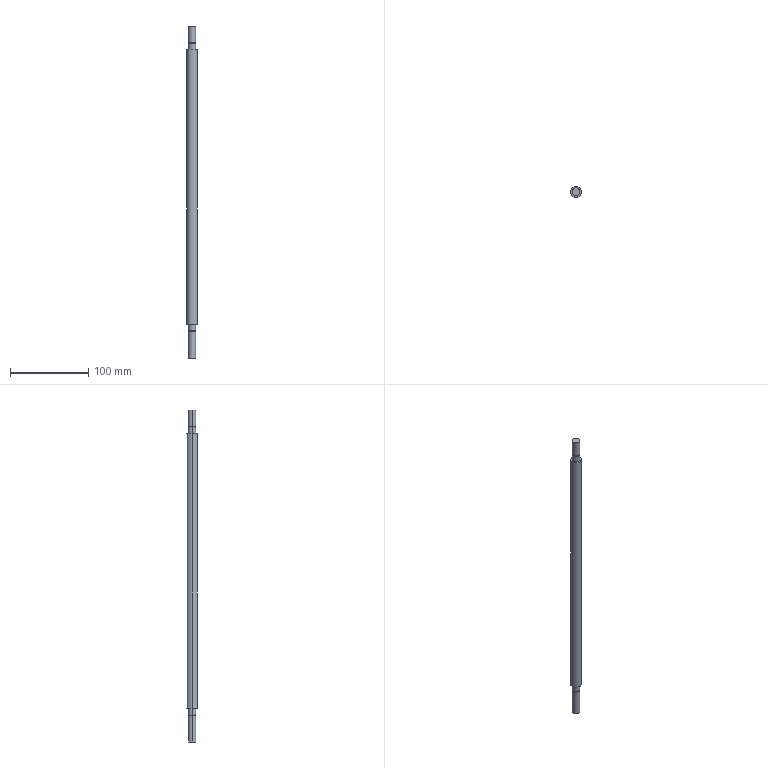Part | STEP file | 602-09-0047 | 1 solid | 24 faces | box 14 x 14 x 425 mm | volume 59824 mm3 | cylinder 14 | plane 10 | commonest cylinder face diameters 10 x8 9.6 x4 14 x2
STEP:
#1=CARTESIAN_POINT('',(0.,0.,0.));
#2=DIRECTION('',(0.,0.,1.));
#3=DIRECTION('',(1.,0.,0.));
#4=AXIS2_PLACEMENT_3D('',#1,#2,#3);
#5=CARTESIAN_POINT('',(-5.,0.,-43.));
#6=VERTEX_POINT('',#5);
#7=CARTESIAN_POINT('',(-3.,4.,-43.));
#8=VERTEX_POINT('',#7);
#9=CARTESIAN_POINT('',(0.,0.,-43.));
#10=DIRECTION('',(0.,0.,-1.));
#11=DIRECTION('',(-1.,0.,0.));
#12=AXIS2_PLACEMENT_3D('',#9,#10,#11);
#13=CIRCLE('',#12,5.);
#14=CARTESIAN_POINT('',(0.,0.,-43.));
#15=DIRECTION('',(0.,0.,1.));
#16=DIRECTION('',(1.,0.,0.));
#17=AXIS2_PLACEMENT_3D('',#14,#15,#16);
#18=CYLINDRICAL_SURFACE('',#17,5.);
#19=CARTESIAN_POINT('',(3.142,0.));
#20=DIRECTION('',(-1.,0.));
#21=VECTOR('',#20,1.);
#22=LINE('',#19,#21);
#23=(GEOMETRIC_REPRESENTATION_CONTEXT(2)PARAMETRIC_REPRESENTATION_CONTEXT()REPRESENTATION_CONTEXT('',''));
#24=DEFINITIONAL_REPRESENTATION('',(#22),#23);
#25=PCURVE('',#18,#24);
#26=CARTESIAN_POINT('',(0.,0.,-43.));
#27=DIRECTION('',(0.,0.,-1.));
#28=DIRECTION('',(-1.,0.,0.));
#29=AXIS2_PLACEMENT_3D('',#26,#27,#28);
#30=PLANE('',#29);
#31=CARTESIAN_POINT('',(0.,0.));
#32=DIRECTION('',(1.,0.));
#33=AXIS2_PLACEMENT_2D('',#31,#32);
#34=CIRCLE('',#33,5.);
#35=(GEOMETRIC_REPRESENTATION_CONTEXT(2)PARAMETRIC_REPRESENTATION_CONTEXT()REPRESENTATION_CONTEXT('',''));
#36=DEFINITIONAL_REPRESENTATION('',(#34),#35);
#37=PCURVE('',#30,#36);
#38=SURFACE_CURVE('',#13,(#25,#37),.PCURVE_S1.);
#39=EDGE_CURVE('',#6,#8,#38,.T.);
#40=ORIENTED_EDGE('',*,*,#39,.F.);
#41=CARTESIAN_POINT('',(-5.,0.,-9.1));
#42=VERTEX_POINT('',#41);
#43=CARTESIAN_POINT('',(-5.,0.,-43.));
#44=DIRECTION('',(0.,0.,1.));
#45=VECTOR('',#44,1.);
#46=LINE('',#43,#45);
#47=CARTESIAN_POINT('',(3.142,0.));
#48=DIRECTION('',(0.,1.));
#49=VECTOR('',#48,1.);
#50=LINE('',#47,#49);
#51=(GEOMETRIC_REPRESENTATION_CONTEXT(2)PARAMETRIC_REPRESENTATION_CONTEXT()REPRESENTATION_CONTEXT('',''));
#52=DEFINITIONAL_REPRESENTATION('',(#50),#51);
#53=PCURVE('',#18,#52);
#54=CARTESIAN_POINT('',(0.,0.,-43.));
#55=DIRECTION('',(0.,0.,1.));
#56=DIRECTION('',(1.,0.,0.));
#57=AXIS2_PLACEMENT_3D('',#54,#55,#56);
#58=CYLINDRICAL_SURFACE('',#57,5.);
#59=CARTESIAN_POINT('',(3.142,0.));
#60=DIRECTION('',(0.,1.));
#61=VECTOR('',#60,1.);
#62=LINE('',#59,#61);
#63=(GEOMETRIC_REPRESENTATION_CONTEXT(2)PARAMETRIC_REPRESENTATION_CONTEXT()REPRESENTATION_CONTEXT('',''));
#64=DEFINITIONAL_REPRESENTATION('',(#62),#63);
#65=PCURVE('',#58,#64);
#66=SURFACE_CURVE('',#46,(#53,#65),.PCURVE_S1.);
#67=EDGE_CURVE('',#6,#42,#66,.T.);
#68=ORIENTED_EDGE('',*,*,#67,.T.);
#69=CARTESIAN_POINT('',(5.,0.,-9.1));
#70=VERTEX_POINT('',#69);
#71=CARTESIAN_POINT('',(0.,0.,-9.1));
#72=DIRECTION('',(0.,0.,-1.));
#73=DIRECTION('',(-1.,0.,0.));
#74=AXIS2_PLACEMENT_3D('',#71,#72,#73);
#75=CIRCLE('',#74,5.);
#76=CARTESIAN_POINT('',(3.142,33.9));
#77=DIRECTION('',(-1.,0.));
#78=VECTOR('',#77,1.);
#79=LINE('',#76,#78);
#80=(GEOMETRIC_REPRESENTATION_CONTEXT(2)PARAMETRIC_REPRESENTATION_CONTEXT()REPRESENTATION_CONTEXT('',''));
#81=DEFINITIONAL_REPRESENTATION('',(#79),#80);
#82=PCURVE('',#18,#81);
#83=CARTESIAN_POINT('',(0.,0.,-9.1));
#84=DIRECTION('',(0.,0.,-1.));
#85=DIRECTION('',(-1.,0.,0.));
#86=AXIS2_PLACEMENT_3D('',#83,#84,#85);
#87=PLANE('',#86);
#88=CARTESIAN_POINT('',(0.,0.));
#89=DIRECTION('',(1.,0.));
#90=AXIS2_PLACEMENT_2D('',#88,#89);
#91=CIRCLE('',#90,5.);
#92=(GEOMETRIC_REPRESENTATION_CONTEXT(2)PARAMETRIC_REPRESENTATION_CONTEXT()REPRESENTATION_CONTEXT('',''));
#93=DEFINITIONAL_REPRESENTATION('',(#91),#92);
#94=PCURVE('',#87,#93);
#95=SURFACE_CURVE('',#75,(#82,#94),.PCURVE_S1.);
#96=EDGE_CURVE('',#42,#70,#95,.T.);
#97=ORIENTED_EDGE('',*,*,#96,.T.);
#98=CARTESIAN_POINT('',(5.,0.,-43.));
#99=VERTEX_POINT('',#98);
#100=CARTESIAN_POINT('',(5.,0.,-43.));
#101=DIRECTION('',(0.,0.,1.));
#102=VECTOR('',#101,1.);
#103=LINE('',#100,#102);
#104=CARTESIAN_POINT('',(0.,0.));
#105=DIRECTION('',(0.,1.));
#106=VECTOR('',#105,1.);
#107=LINE('',#104,#106);
#108=(GEOMETRIC_REPRESENTATION_CONTEXT(2)PARAMETRIC_REPRESENTATION_CONTEXT()REPRESENTATION_CONTEXT('',''));
#109=DEFINITIONAL_REPRESENTATION('',(#107),#108);
#110=PCURVE('',#18,#109);
#111=CARTESIAN_POINT('',(6.283,0.));
#112=DIRECTION('',(0.,1.));
#113=VECTOR('',#112,1.);
#114=LINE('',#111,#113);
#115=(GEOMETRIC_REPRESENTATION_CONTEXT(2)PARAMETRIC_REPRESENTATION_CONTEXT()REPRESENTATION_CONTEXT('',''));
#116=DEFINITIONAL_REPRESENTATION('',(#114),#115);
#117=PCURVE('',#58,#116);
#118=SURFACE_CURVE('',#103,(#110,#117),.PCURVE_S1.);
#119=EDGE_CURVE('',#99,#70,#118,.T.);
#120=ORIENTED_EDGE('',*,*,#119,.F.);
#121=CARTESIAN_POINT('',(3.,4.,-43.));
#122=VERTEX_POINT('',#121);
#123=CARTESIAN_POINT('',(0.,0.,-43.));
#124=DIRECTION('',(0.,0.,-1.));
#125=DIRECTION('',(-1.,0.,0.));
#126=AXIS2_PLACEMENT_3D('',#123,#124,#125);
#127=CIRCLE('',#126,5.);
#128=CARTESIAN_POINT('',(3.142,0.));
#129=DIRECTION('',(-1.,0.));
#130=VECTOR('',#129,1.);
#131=LINE('',#128,#130);
#132=(GEOMETRIC_REPRESENTATION_CONTEXT(2)PARAMETRIC_REPRESENTATION_CONTEXT()REPRESENTATION_CONTEXT('',''));
#133=DEFINITIONAL_REPRESENTATION('',(#131),#132);
#134=PCURVE('',#18,#133);
#135=CARTESIAN_POINT('',(0.,0.));
#136=DIRECTION('',(1.,0.));
#137=AXIS2_PLACEMENT_2D('',#135,#136);
#138=CIRCLE('',#137,5.);
#139=(GEOMETRIC_REPRESENTATION_CONTEXT(2)PARAMETRIC_REPRESENTATION_CONTEXT()REPRESENTATION_CONTEXT('',''));
#140=DEFINITIONAL_REPRESENTATION('',(#138),#139);
#141=PCURVE('',#30,#140);
#142=SURFACE_CURVE('',#127,(#134,#141),.PCURVE_S1.);
#143=EDGE_CURVE('',#122,#99,#142,.T.);
#144=ORIENTED_EDGE('',*,*,#143,.F.);
#145=CARTESIAN_POINT('',(3.,4.,-23.));
#146=VERTEX_POINT('',#145);
#147=CARTESIAN_POINT('',(3.,4.,-23.));
#148=DIRECTION('',(0.,0.,-1.));
#149=VECTOR('',#148,1.);
#150=LINE('',#147,#149);
#151=CARTESIAN_POINT('',(0.9273,20.));
#152=DIRECTION('',(0.,-1.));
#153=VECTOR('',#152,1.);
#154=LINE('',#151,#153);
#155=(GEOMETRIC_REPRESENTATION_CONTEXT(2)PARAMETRIC_REPRESENTATION_CONTEXT()REPRESENTATION_CONTEXT('',''));
#156=DEFINITIONAL_REPRESENTATION('',(#154),#155);
#157=PCURVE('',#18,#156);
#158=CARTESIAN_POINT('',(3.,4.,-23.));
#159=DIRECTION('',(0.,-1.,0.));
#160=DIRECTION('',(0.,0.,-1.));
#161=AXIS2_PLACEMENT_3D('',#158,#159,#160);
#162=PLANE('',#161);
#163=CARTESIAN_POINT('',(0.,0.));
#164=DIRECTION('',(1.,0.));
#165=VECTOR('',#164,1.);
#166=LINE('',#163,#165);
#167=(GEOMETRIC_REPRESENTATION_CONTEXT(2)PARAMETRIC_REPRESENTATION_CONTEXT()REPRESENTATION_CONTEXT('',''));
#168=DEFINITIONAL_REPRESENTATION('',(#166),#167);
#169=PCURVE('',#162,#168);
#170=SURFACE_CURVE('',#150,(#157,#169),.PCURVE_S1.);
#171=EDGE_CURVE('',#146,#122,#170,.T.);
#172=ORIENTED_EDGE('',*,*,#171,.F.);
#173=CARTESIAN_POINT('',(-3.,4.,-23.));
#174=VERTEX_POINT('',#173);
#175=CARTESIAN_POINT('',(0.,0.,-23.));
#176=DIRECTION('',(0.,0.,-1.));
#177=DIRECTION('',(-1.,0.,0.));
#178=AXIS2_PLACEMENT_3D('',#175,#176,#177);
#179=CIRCLE('',#178,5.);
#180=CARTESIAN_POINT('',(3.142,20.));
#181=DIRECTION('',(-1.,0.));
#182=VECTOR('',#181,1.);
#183=LINE('',#180,#182);
#184=(GEOMETRIC_REPRESENTATION_CONTEXT(2)PARAMETRIC_REPRESENTATION_CONTEXT()REPRESENTATION_CONTEXT('',''));
#185=DEFINITIONAL_REPRESENTATION('',(#183),#184);
#186=PCURVE('',#18,#185);
#187=CARTESIAN_POINT('',(0.,0.,-23.));
#188=DIRECTION('',(0.,0.,-1.));
#189=DIRECTION('',(-1.,0.,0.));
#190=AXIS2_PLACEMENT_3D('',#187,#188,#189);
#191=PLANE('',#190);
#192=CARTESIAN_POINT('',(0.,0.));
#193=DIRECTION('',(1.,0.));
#194=AXIS2_PLACEMENT_2D('',#192,#193);
#195=CIRCLE('',#194,5.);
#196=(GEOMETRIC_REPRESENTATION_CONTEXT(2)PARAMETRIC_REPRESENTATION_CONTEXT()REPRESENTATION_CONTEXT('',''));
#197=DEFINITIONAL_REPRESENTATION('',(#195),#196);
#198=PCURVE('',#191,#197);
#199=SURFACE_CURVE('',#179,(#186,#198),.PCURVE_S1.);
#200=EDGE_CURVE('',#174,#146,#199,.T.);
#201=ORIENTED_EDGE('',*,*,#200,.F.);
#202=CARTESIAN_POINT('',(-3.,4.,-23.));
#203=DIRECTION('',(0.,0.,-1.));
#204=VECTOR('',#203,1.);
#205=LINE('',#202,#204);
#206=CARTESIAN_POINT('',(2.214,20.));
#207=DIRECTION('',(0.,-1.));
#208=VECTOR('',#207,1.);
#209=LINE('',#206,#208);
#210=(GEOMETRIC_REPRESENTATION_CONTEXT(2)PARAMETRIC_REPRESENTATION_CONTEXT()REPRESENTATION_CONTEXT('',''));
#211=DEFINITIONAL_REPRESENTATION('',(#209),#210);
#212=PCURVE('',#18,#211);
#213=CARTESIAN_POINT('',(0.,-6.));
#214=DIRECTION('',(1.,0.));
#215=VECTOR('',#214,1.);
#216=LINE('',#213,#215);
#217=(GEOMETRIC_REPRESENTATION_CONTEXT(2)PARAMETRIC_REPRESENTATION_CONTEXT()REPRESENTATION_CONTEXT('',''));
#218=DEFINITIONAL_REPRESENTATION('',(#216),#217);
#219=PCURVE('',#162,#218);
#220=SURFACE_CURVE('',#205,(#212,#219),.PCURVE_S1.);
#221=EDGE_CURVE('',#174,#8,#220,.T.);
#222=ORIENTED_EDGE('',*,*,#221,.T.);
#223=EDGE_LOOP('',(#40,#68,#97,#120,#144,#172,#201,#222));
#224=FACE_BOUND('',#223,.T.);
#225=ADVANCED_FACE('',(#224),#18,.T.);
#226=CARTESIAN_POINT('',(-4.8,0.,-9.1));
#227=VERTEX_POINT('',#226);
#228=CARTESIAN_POINT('',(4.8,0.,-9.1));
#229=VERTEX_POINT('',#228);
#230=CARTESIAN_POINT('',(0.,0.,-9.1));
#231=DIRECTION('',(0.,0.,-1.));
#232=DIRECTION('',(-1.,0.,0.));
#233=AXIS2_PLACEMENT_3D('',#230,#231,#232);
#234=CIRCLE('',#233,4.8);
#235=CARTESIAN_POINT('',(0.,0.,-9.1));
#236=DIRECTION('',(0.,0.,1.));
#237=DIRECTION('',(1.,0.,0.));
#238=AXIS2_PLACEMENT_3D('',#235,#236,#237);
#239=CYLINDRICAL_SURFACE('',#238,4.8);
#240=CARTESIAN_POINT('',(3.142,0.));
#241=DIRECTION('',(-1.,0.));
#242=VECTOR('',#241,1.);
#243=LINE('',#240,#242);
#244=(GEOMETRIC_REPRESENTATION_CONTEXT(2)PARAMETRIC_REPRESENTATION_CONTEXT()REPRESENTATION_CONTEXT('',''));
#245=DEFINITIONAL_REPRESENTATION('',(#243),#244);
#246=PCURVE('',#239,#245);
#247=CARTESIAN_POINT('',(0.,0.));
#248=DIRECTION('',(1.,0.));
#249=AXIS2_PLACEMENT_2D('',#247,#248);
#250=CIRCLE('',#249,4.8);
#251=(GEOMETRIC_REPRESENTATION_CONTEXT(2)PARAMETRIC_REPRESENTATION_CONTEXT()REPRESENTATION_CONTEXT('',''));
#252=DEFINITIONAL_REPRESENTATION('',(#250),#251);
#253=PCURVE('',#87,#252);
#254=SURFACE_CURVE('',#234,(#246,#253),.PCURVE_S1.);
#255=EDGE_CURVE('',#227,#229,#254,.T.);
#256=ORIENTED_EDGE('',*,*,#255,.F.);
#257=CARTESIAN_POINT('',(-4.8,0.,-8.));
#258=VERTEX_POINT('',#257);
#259=CARTESIAN_POINT('',(-4.8,0.,-9.1));
#260=DIRECTION('',(0.,0.,1.));
#261=VECTOR('',#260,1.);
#262=LINE('',#259,#261);
#263=CARTESIAN_POINT('',(3.142,0.));
#264=DIRECTION('',(0.,1.));
#265=VECTOR('',#264,1.);
#266=LINE('',#263,#265);
#267=(GEOMETRIC_REPRESENTATION_CONTEXT(2)PARAMETRIC_REPRESENTATION_CONTEXT()REPRESENTATION_CONTEXT('',''));
#268=DEFINITIONAL_REPRESENTATION('',(#266),#267);
#269=PCURVE('',#239,#268);
#270=CARTESIAN_POINT('',(0.,0.,-9.1));
#271=DIRECTION('',(0.,0.,1.));
#272=DIRECTION('',(1.,0.,0.));
#273=AXIS2_PLACEMENT_3D('',#270,#271,#272);
#274=CYLINDRICAL_SURFACE('',#273,4.8);
#275=CARTESIAN_POINT('',(3.142,0.));
#276=DIRECTION('',(0.,1.));
#277=VECTOR('',#276,1.);
#278=LINE('',#275,#277);
#279=(GEOMETRIC_REPRESENTATION_CONTEXT(2)PARAMETRIC_REPRESENTATION_CONTEXT()REPRESENTATION_CONTEXT('',''));
#280=DEFINITIONAL_REPRESENTATION('',(#278),#279);
#281=PCURVE('',#274,#280);
#282=SURFACE_CURVE('',#262,(#269,#281),.PCURVE_S1.);
#283=EDGE_CURVE('',#227,#258,#282,.T.);
#284=ORIENTED_EDGE('',*,*,#283,.T.);
#285=CARTESIAN_POINT('',(4.8,0.,-8.));
#286=VERTEX_POINT('',#285);
#287=CARTESIAN_POINT('',(0.,0.,-8.));
#288=DIRECTION('',(0.,0.,-1.));
#289=DIRECTION('',(-1.,0.,0.));
#290=AXIS2_PLACEMENT_3D('',#287,#288,#289);
#291=CIRCLE('',#290,4.8);
#292=CARTESIAN_POINT('',(3.142,1.1));
#293=DIRECTION('',(-1.,0.));
#294=VECTOR('',#293,1.);
#295=LINE('',#292,#294);
#296=(GEOMETRIC_REPRESENTATION_CONTEXT(2)PARAMETRIC_REPRESENTATION_CONTEXT()REPRESENTATION_CONTEXT('',''));
#297=DEFINITIONAL_REPRESENTATION('',(#295),#296);
#298=PCURVE('',#239,#297);
#299=CARTESIAN_POINT('',(0.,0.,-8.));
#300=DIRECTION('',(0.,0.,-1.));
#301=DIRECTION('',(-1.,0.,0.));
#302=AXIS2_PLACEMENT_3D('',#299,#300,#301);
#303=PLANE('',#302);
#304=CARTESIAN_POINT('',(0.,0.));
#305=DIRECTION('',(1.,0.));
#306=AXIS2_PLACEMENT_2D('',#304,#305);
#307=CIRCLE('',#306,4.8);
#308=(GEOMETRIC_REPRESENTATION_CONTEXT(2)PARAMETRIC_REPRESENTATION_CONTEXT()REPRESENTATION_CONTEXT('',''));
#309=DEFINITIONAL_REPRESENTATION('',(#307),#308);
#310=PCURVE('',#303,#309);
#311=SURFACE_CURVE('',#291,(#298,#310),.PCURVE_S1.);
#312=EDGE_CURVE('',#258,#286,#311,.T.);
#313=ORIENTED_EDGE('',*,*,#312,.T.);
#314=CARTESIAN_POINT('',(4.8,0.,-9.1));
#315=DIRECTION('',(0.,0.,1.));
#316=VECTOR('',#315,1.);
#317=LINE('',#314,#316);
#318=CARTESIAN_POINT('',(0.,0.));
#319=DIRECTION('',(0.,1.));
#320=VECTOR('',#319,1.);
#321=LINE('',#318,#320);
#322=(GEOMETRIC_REPRESENTATION_CONTEXT(2)PARAMETRIC_REPRESENTATION_CONTEXT()REPRESENTATION_CONTEXT('',''));
#323=DEFINITIONAL_REPRESENTATION('',(#321),#322);
#324=PCURVE('',#239,#323);
#325=CARTESIAN_POINT('',(6.283,0.));
#326=DIRECTION('',(0.,1.));
#327=VECTOR('',#326,1.);
#328=LINE('',#325,#327);
#329=(GEOMETRIC_REPRESENTATION_CONTEXT(2)PARAMETRIC_REPRESENTATION_CONTEXT()REPRESENTATION_CONTEXT('',''));
#330=DEFINITIONAL_REPRESENTATION('',(#328),#329);
#331=PCURVE('',#274,#330);
#332=SURFACE_CURVE('',#317,(#324,#331),.PCURVE_S1.);
#333=EDGE_CURVE('',#229,#286,#332,.T.);
#334=ORIENTED_EDGE('',*,*,#333,.F.);
#335=EDGE_LOOP('',(#256,#284,#313,#334));
#336=FACE_BOUND('',#335,.T.);
#337=ADVANCED_FACE('',(#336),#239,.T.);
#338=CARTESIAN_POINT('',(5.,0.,382.));
#339=VERTEX_POINT('',#338);
#340=CARTESIAN_POINT('',(-5.,0.,382.));
#341=VERTEX_POINT('',#340);
#342=CARTESIAN_POINT('',(0.,0.,382.));
#343=DIRECTION('',(0.,0.,1.));
#344=DIRECTION('',(1.,0.,0.));
#345=AXIS2_PLACEMENT_3D('',#342,#343,#344);
#346=CIRCLE('',#345,5.);
#347=CARTESIAN_POINT('',(0.,0.,382.));
#348=DIRECTION('',(0.,0.,-1.));
#349=DIRECTION('',(-1.,0.,0.));
#350=AXIS2_PLACEMENT_3D('',#347,#348,#349);
#351=CYLINDRICAL_SURFACE('',#350,5.);
#352=CARTESIAN_POINT('',(3.142,0.));
#353=DIRECTION('',(-1.,0.));
#354=VECTOR('',#353,1.);
#355=LINE('',#352,#354);
#356=(GEOMETRIC_REPRESENTATION_CONTEXT(2)PARAMETRIC_REPRESENTATION_CONTEXT()REPRESENTATION_CONTEXT('',''));
#357=DEFINITIONAL_REPRESENTATION('',(#355),#356);
#358=PCURVE('',#351,#357);
#359=CARTESIAN_POINT('',(0.,0.,382.));
#360=DIRECTION('',(0.,0.,1.));
#361=DIRECTION('',(1.,0.,0.));
#362=AXIS2_PLACEMENT_3D('',#359,#360,#361);
#363=PLANE('',#362);
#364=CARTESIAN_POINT('',(0.,0.));
#365=DIRECTION('',(1.,0.));
#366=AXIS2_PLACEMENT_2D('',#364,#365);
#367=CIRCLE('',#366,5.);
#368=(GEOMETRIC_REPRESENTATION_CONTEXT(2)PARAMETRIC_REPRESENTATION_CONTEXT()REPRESENTATION_CONTEXT('',''));
#369=DEFINITIONAL_REPRESENTATION('',(#367),#368);
#370=PCURVE('',#363,#369);
#371=SURFACE_CURVE('',#346,(#358,#370),.PCURVE_S1.);
#372=EDGE_CURVE('',#339,#341,#371,.T.);
#373=ORIENTED_EDGE('',*,*,#372,.F.);
#374=CARTESIAN_POINT('',(5.,0.,361.1));
#375=VERTEX_POINT('',#374);
#376=CARTESIAN_POINT('',(5.,0.,382.));
#377=DIRECTION('',(0.,0.,-1.));
#378=VECTOR('',#377,1.);
#379=LINE('',#376,#378);
#380=CARTESIAN_POINT('',(3.142,0.));
#381=DIRECTION('',(0.,1.));
#382=VECTOR('',#381,1.);
#383=LINE('',#380,#382);
#384=(GEOMETRIC_REPRESENTATION_CONTEXT(2)PARAMETRIC_REPRESENTATION_CONTEXT()REPRESENTATION_CONTEXT('',''));
#385=DEFINITIONAL_REPRESENTATION('',(#383),#384);
#386=PCURVE('',#351,#385);
#387=CARTESIAN_POINT('',(0.,0.,382.));
#388=DIRECTION('',(0.,0.,-1.));
#389=DIRECTION('',(-1.,0.,0.));
#390=AXIS2_PLACEMENT_3D('',#387,#388,#389);
#391=CYLINDRICAL_SURFACE('',#390,5.);
#392=CARTESIAN_POINT('',(3.142,0.));
#393=DIRECTION('',(0.,1.));
#394=VECTOR('',#393,1.);
#395=LINE('',#392,#394);
#396=(GEOMETRIC_REPRESENTATION_CONTEXT(2)PARAMETRIC_REPRESENTATION_CONTEXT()REPRESENTATION_CONTEXT('',''));
#397=DEFINITIONAL_REPRESENTATION('',(#395),#396);
#398=PCURVE('',#391,#397);
#399=SURFACE_CURVE('',#379,(#386,#398),.PCURVE_S1.);
#400=EDGE_CURVE('',#339,#375,#399,.T.);
#401=ORIENTED_EDGE('',*,*,#400,.T.);
#402=CARTESIAN_POINT('',(-5.,0.,361.1));
#403=VERTEX_POINT('',#402);
#404=CARTESIAN_POINT('',(0.,0.,361.1));
#405=DIRECTION('',(0.,0.,1.));
#406=DIRECTION('',(1.,0.,0.));
#407=AXIS2_PLACEMENT_3D('',#404,#405,#406);
#408=CIRCLE('',#407,5.);
#409=CARTESIAN_POINT('',(3.142,20.9));
#410=DIRECTION('',(-1.,0.));
#411=VECTOR('',#410,1.);
#412=LINE('',#409,#411);
#413=(GEOMETRIC_REPRESENTATION_CONTEXT(2)PARAMETRIC_REPRESENTATION_CONTEXT()REPRESENTATION_CONTEXT('',''));
#414=DEFINITIONAL_REPRESENTATION('',(#412),#413);
#415=PCURVE('',#351,#414);
#416=CARTESIAN_POINT('',(0.,0.,361.1));
#417=DIRECTION('',(0.,0.,1.));
#418=DIRECTION('',(1.,0.,0.));
#419=AXIS2_PLACEMENT_3D('',#416,#417,#418);
#420=PLANE('',#419);
#421=CARTESIAN_POINT('',(0.,0.));
#422=DIRECTION('',(1.,0.));
#423=AXIS2_PLACEMENT_2D('',#421,#422);
#424=CIRCLE('',#423,5.);
#425=(GEOMETRIC_REPRESENTATION_CONTEXT(2)PARAMETRIC_REPRESENTATION_CONTEXT()REPRESENTATION_CONTEXT('',''));
#426=DEFINITIONAL_REPRESENTATION('',(#424),#425);
#427=PCURVE('',#420,#426);
#428=SURFACE_CURVE('',#408,(#415,#427),.PCURVE_S1.);
#429=EDGE_CURVE('',#375,#403,#428,.T.);
#430=ORIENTED_EDGE('',*,*,#429,.T.);
#431=CARTESIAN_POINT('',(-5.,0.,382.));
#432=DIRECTION('',(0.,0.,-1.));
#433=VECTOR('',#432,1.);
#434=LINE('',#431,#433);
#435=CARTESIAN_POINT('',(0.,0.));
#436=DIRECTION('',(0.,1.));
#437=VECTOR('',#436,1.);
#438=LINE('',#435,#437);
#439=(GEOMETRIC_REPRESENTATION_CONTEXT(2)PARAMETRIC_REPRESENTATION_CONTEXT()REPRESENTATION_CONTEXT('',''));
#440=DEFINITIONAL_REPRESENTATION('',(#438),#439);
#441=PCURVE('',#351,#440);
#442=CARTESIAN_POINT('',(6.283,0.));
#443=DIRECTION('',(0.,1.));
#444=VECTOR('',#443,1.);
#445=LINE('',#442,#444);
#446=(GEOMETRIC_REPRESENTATION_CONTEXT(2)PARAMETRIC_REPRESENTATION_CONTEXT()REPRESENTATION_CONTEXT('',''));
#447=DEFINITIONAL_REPRESENTATION('',(#445),#446);
#448=PCURVE('',#391,#447);
#449=SURFACE_CURVE('',#434,(#441,#448),.PCURVE_S1.);
#450=EDGE_CURVE('',#341,#403,#449,.T.);
#451=ORIENTED_EDGE('',*,*,#450,.F.);
#452=EDGE_LOOP('',(#373,#401,#430,#451));
#453=FACE_BOUND('',#452,.T.);
#454=ADVANCED_FACE('',(#453),#351,.T.);
#455=CARTESIAN_POINT('',(4.8,0.,361.1));
#456=VERTEX_POINT('',#455);
#457=CARTESIAN_POINT('',(-4.8,0.,361.1));
#458=VERTEX_POINT('',#457);
#459=CARTESIAN_POINT('',(0.,0.,361.1));
#460=DIRECTION('',(0.,0.,1.));
#461=DIRECTION('',(1.,0.,0.));
#462=AXIS2_PLACEMENT_3D('',#459,#460,#461);
#463=CIRCLE('',#462,4.8);
#464=CARTESIAN_POINT('',(0.,0.,361.1));
#465=DIRECTION('',(0.,0.,-1.));
#466=DIRECTION('',(-1.,0.,0.));
#467=AXIS2_PLACEMENT_3D('',#464,#465,#466);
#468=CYLINDRICAL_SURFACE('',#467,4.8);
#469=CARTESIAN_POINT('',(3.142,0.));
#470=DIRECTION('',(-1.,0.));
#471=VECTOR('',#470,1.);
#472=LINE('',#469,#471);
#473=(GEOMETRIC_REPRESENTATION_CONTEXT(2)PARAMETRIC_REPRESENTATION_CONTEXT()REPRESENTATION_CONTEXT('',''));
#474=DEFINITIONAL_REPRESENTATION('',(#472),#473);
#475=PCURVE('',#468,#474);
#476=CARTESIAN_POINT('',(0.,0.));
#477=DIRECTION('',(1.,0.));
#478=AXIS2_PLACEMENT_2D('',#476,#477);
#479=CIRCLE('',#478,4.8);
#480=(GEOMETRIC_REPRESENTATION_CONTEXT(2)PARAMETRIC_REPRESENTATION_CONTEXT()REPRESENTATION_CONTEXT('',''));
#481=DEFINITIONAL_REPRESENTATION('',(#479),#480);
#482=PCURVE('',#420,#481);
#483=SURFACE_CURVE('',#463,(#475,#482),.PCURVE_S1.);
#484=EDGE_CURVE('',#456,#458,#483,.T.);
#485=ORIENTED_EDGE('',*,*,#484,.F.);
#486=CARTESIAN_POINT('',(4.8,0.,360.));
#487=VERTEX_POINT('',#486);
#488=CARTESIAN_POINT('',(4.8,0.,361.1));
#489=DIRECTION('',(0.,0.,-1.));
#490=VECTOR('',#489,1.);
#491=LINE('',#488,#490);
#492=CARTESIAN_POINT('',(3.142,0.));
#493=DIRECTION('',(0.,1.));
#494=VECTOR('',#493,1.);
#495=LINE('',#492,#494);
#496=(GEOMETRIC_REPRESENTATION_CONTEXT(2)PARAMETRIC_REPRESENTATION_CONTEXT()REPRESENTATION_CONTEXT('',''));
#497=DEFINITIONAL_REPRESENTATION('',(#495),#496);
#498=PCURVE('',#468,#497);
#499=CARTESIAN_POINT('',(0.,0.,361.1));
#500=DIRECTION('',(0.,0.,-1.));
#501=DIRECTION('',(-1.,0.,0.));
#502=AXIS2_PLACEMENT_3D('',#499,#500,#501);
#503=CYLINDRICAL_SURFACE('',#502,4.8);
#504=CARTESIAN_POINT('',(3.142,0.));
#505=DIRECTION('',(0.,1.));
#506=VECTOR('',#505,1.);
#507=LINE('',#504,#506);
#508=(GEOMETRIC_REPRESENTATION_CONTEXT(2)PARAMETRIC_REPRESENTATION_CONTEXT()REPRESENTATION_CONTEXT('',''));
#509=DEFINITIONAL_REPRESENTATION('',(#507),#508);
#510=PCURVE('',#503,#509);
#511=SURFACE_CURVE('',#491,(#498,#510),.PCURVE_S1.);
#512=EDGE_CURVE('',#456,#487,#511,.T.);
#513=ORIENTED_EDGE('',*,*,#512,.T.);
#514=CARTESIAN_POINT('',(-4.8,0.,360.));
#515=VERTEX_POINT('',#514);
#516=CARTESIAN_POINT('',(0.,0.,360.));
#517=DIRECTION('',(0.,0.,1.));
#518=DIRECTION('',(1.,0.,0.));
#519=AXIS2_PLACEMENT_3D('',#516,#517,#518);
#520=CIRCLE('',#519,4.8);
#521=CARTESIAN_POINT('',(3.142,1.1));
#522=DIRECTION('',(-1.,0.));
#523=VECTOR('',#522,1.);
#524=LINE('',#521,#523);
#525=(GEOMETRIC_REPRESENTATION_CONTEXT(2)PARAMETRIC_REPRESENTATION_CONTEXT()REPRESENTATION_CONTEXT('',''));
#526=DEFINITIONAL_REPRESENTATION('',(#524),#525);
#527=PCURVE('',#468,#526);
#528=CARTESIAN_POINT('',(0.,0.,360.));
#529=DIRECTION('',(0.,0.,1.));
#530=DIRECTION('',(1.,0.,0.));
#531=AXIS2_PLACEMENT_3D('',#528,#529,#530);
#532=PLANE('',#531);
#533=CARTESIAN_POINT('',(0.,0.));
#534=DIRECTION('',(1.,0.));
#535=AXIS2_PLACEMENT_2D('',#533,#534);
#536=CIRCLE('',#535,4.8);
#537=(GEOMETRIC_REPRESENTATION_CONTEXT(2)PARAMETRIC_REPRESENTATION_CONTEXT()REPRESENTATION_CONTEXT('',''));
#538=DEFINITIONAL_REPRESENTATION('',(#536),#537);
#539=PCURVE('',#532,#538);
#540=SURFACE_CURVE('',#520,(#527,#539),.PCURVE_S1.);
#541=EDGE_CURVE('',#487,#515,#540,.T.);
#542=ORIENTED_EDGE('',*,*,#541,.T.);
#543=CARTESIAN_POINT('',(-4.8,0.,361.1));
#544=DIRECTION('',(0.,0.,-1.));
#545=VECTOR('',#544,1.);
#546=LINE('',#543,#545);
#547=CARTESIAN_POINT('',(0.,0.));
#548=DIRECTION('',(0.,1.));
#549=VECTOR('',#548,1.);
#550=LINE('',#547,#549);
#551=(GEOMETRIC_REPRESENTATION_CONTEXT(2)PARAMETRIC_REPRESENTATION_CONTEXT()REPRESENTATION_CONTEXT('',''));
#552=DEFINITIONAL_REPRESENTATION('',(#550),#551);
#553=PCURVE('',#468,#552);
#554=CARTESIAN_POINT('',(6.283,0.));
#555=DIRECTION('',(0.,1.));
#556=VECTOR('',#555,1.);
#557=LINE('',#554,#556);
#558=(GEOMETRIC_REPRESENTATION_CONTEXT(2)PARAMETRIC_REPRESENTATION_CONTEXT()REPRESENTATION_CONTEXT('',''));
#559=DEFINITIONAL_REPRESENTATION('',(#557),#558);
#560=PCURVE('',#503,#559);
#561=SURFACE_CURVE('',#546,(#553,#560),.PCURVE_S1.);
#562=EDGE_CURVE('',#458,#515,#561,.T.);
#563=ORIENTED_EDGE('',*,*,#562,.F.);
#564=EDGE_LOOP('',(#485,#513,#542,#563));
#565=FACE_BOUND('',#564,.T.);
#566=ADVANCED_FACE('',(#565),#468,.T.);
#567=CARTESIAN_POINT('',(7.,0.,352.));
#568=VERTEX_POINT('',#567);
#569=CARTESIAN_POINT('',(-7.,0.,352.));
#570=VERTEX_POINT('',#569);
#571=CARTESIAN_POINT('',(0.,0.,352.));
#572=DIRECTION('',(0.,0.,1.));
#573=DIRECTION('',(1.,0.,0.));
#574=AXIS2_PLACEMENT_3D('',#571,#572,#573);
#575=CIRCLE('',#574,7.);
#576=CARTESIAN_POINT('',(0.,0.,352.));
#577=DIRECTION('',(0.,0.,-1.));
#578=DIRECTION('',(-1.,0.,0.));
#579=AXIS2_PLACEMENT_3D('',#576,#577,#578);
#580=CYLINDRICAL_SURFACE('',#579,7.);
#581=CARTESIAN_POINT('',(3.142,0.));
#582=DIRECTION('',(-1.,0.));
#583=VECTOR('',#582,1.);
#584=LINE('',#581,#583);
#585=(GEOMETRIC_REPRESENTATION_CONTEXT(2)PARAMETRIC_REPRESENTATION_CONTEXT()REPRESENTATION_CONTEXT('',''));
#586=DEFINITIONAL_REPRESENTATION('',(#584),#585);
#587=PCURVE('',#580,#586);
#588=CARTESIAN_POINT('',(0.,0.,352.));
#589=DIRECTION('',(0.,0.,1.));
#590=DIRECTION('',(1.,0.,0.));
#591=AXIS2_PLACEMENT_3D('',#588,#589,#590);
#592=PLANE('',#591);
#593=CARTESIAN_POINT('',(0.,0.));
#594=DIRECTION('',(1.,0.));
#595=AXIS2_PLACEMENT_2D('',#593,#594);
#596=CIRCLE('',#595,7.);
#597=(GEOMETRIC_REPRESENTATION_CONTEXT(2)PARAMETRIC_REPRESENTATION_CONTEXT()REPRESENTATION_CONTEXT('',''));
#598=DEFINITIONAL_REPRESENTATION('',(#596),#597);
#599=PCURVE('',#592,#598);
#600=SURFACE_CURVE('',#575,(#587,#599),.PCURVE_S1.);
#601=EDGE_CURVE('',#568,#570,#600,.T.);
#602=ORIENTED_EDGE('',*,*,#601,.F.);
#603=CARTESIAN_POINT('',(7.,0.,0.));
#604=VERTEX_POINT('',#603);
#605=CARTESIAN_POINT('',(7.,0.,352.));
#606=DIRECTION('',(0.,0.,-1.));
#607=VECTOR('',#606,1.);
#608=LINE('',#605,#607);
#609=CARTESIAN_POINT('',(3.142,0.));
#610=DIRECTION('',(0.,1.));
#611=VECTOR('',#610,1.);
#612=LINE('',#609,#611);
#613=(GEOMETRIC_REPRESENTATION_CONTEXT(2)PARAMETRIC_REPRESENTATION_CONTEXT()REPRESENTATION_CONTEXT('',''));
#614=DEFINITIONAL_REPRESENTATION('',(#612),#613);
#615=PCURVE('',#580,#614);
#616=CARTESIAN_POINT('',(0.,0.,352.));
#617=DIRECTION('',(0.,0.,-1.));
#618=DIRECTION('',(-1.,0.,0.));
#619=AXIS2_PLACEMENT_3D('',#616,#617,#618);
#620=CYLINDRICAL_SURFACE('',#619,7.);
#621=CARTESIAN_POINT('',(3.142,0.));
#622=DIRECTION('',(0.,1.));
#623=VECTOR('',#622,1.);
#624=LINE('',#621,#623);
#625=(GEOMETRIC_REPRESENTATION_CONTEXT(2)PARAMETRIC_REPRESENTATION_CONTEXT()REPRESENTATION_CONTEXT('',''));
#626=DEFINITIONAL_REPRESENTATION('',(#624),#625);
#627=PCURVE('',#620,#626);
#628=SURFACE_CURVE('',#608,(#615,#627),.PCURVE_S1.);
#629=EDGE_CURVE('',#568,#604,#628,.T.);
#630=ORIENTED_EDGE('',*,*,#629,.T.);
#631=CARTESIAN_POINT('',(-7.,0.,0.));
#632=VERTEX_POINT('',#631);
#633=CARTESIAN_POINT('',(0.,0.,0.));
#634=DIRECTION('',(0.,0.,1.));
#635=DIRECTION('',(1.,0.,0.));
#636=AXIS2_PLACEMENT_3D('',#633,#634,#635);
#637=CIRCLE('',#636,7.);
#638=CARTESIAN_POINT('',(3.142,352.));
#639=DIRECTION('',(-1.,0.));
#640=VECTOR('',#639,1.);
#641=LINE('',#638,#640);
#642=(GEOMETRIC_REPRESENTATION_CONTEXT(2)PARAMETRIC_REPRESENTATION_CONTEXT()REPRESENTATION_CONTEXT('',''));
#643=DEFINITIONAL_REPRESENTATION('',(#641),#642);
#644=PCURVE('',#580,#643);
#645=CARTESIAN_POINT('',(0.,0.,0.));
#646=DIRECTION('',(0.,0.,1.));
#647=DIRECTION('',(1.,0.,0.));
#648=AXIS2_PLACEMENT_3D('',#645,#646,#647);
#649=PLANE('',#648);
#650=CARTESIAN_POINT('',(0.,0.));
#651=DIRECTION('',(1.,0.));
#652=AXIS2_PLACEMENT_2D('',#650,#651);
#653=CIRCLE('',#652,7.);
#654=(GEOMETRIC_REPRESENTATION_CONTEXT(2)PARAMETRIC_REPRESENTATION_CONTEXT()REPRESENTATION_CONTEXT('',''));
#655=DEFINITIONAL_REPRESENTATION('',(#653),#654);
#656=PCURVE('',#649,#655);
#657=SURFACE_CURVE('',#637,(#644,#656),.PCURVE_S1.);
#658=EDGE_CURVE('',#604,#632,#657,.T.);
#659=ORIENTED_EDGE('',*,*,#658,.T.);
#660=CARTESIAN_POINT('',(-7.,0.,352.));
#661=DIRECTION('',(0.,0.,-1.));
#662=VECTOR('',#661,1.);
#663=LINE('',#660,#662);
#664=CARTESIAN_POINT('',(0.,0.));
#665=DIRECTION('',(0.,1.));
#666=VECTOR('',#665,1.);
#667=LINE('',#664,#666);
#668=(GEOMETRIC_REPRESENTATION_CONTEXT(2)PARAMETRIC_REPRESENTATION_CONTEXT()REPRESENTATION_CONTEXT('',''));
#669=DEFINITIONAL_REPRESENTATION('',(#667),#668);
#670=PCURVE('',#580,#669);
#671=CARTESIAN_POINT('',(6.283,0.));
#672=DIRECTION('',(0.,1.));
#673=VECTOR('',#672,1.);
#674=LINE('',#671,#673);
#675=(GEOMETRIC_REPRESENTATION_CONTEXT(2)PARAMETRIC_REPRESENTATION_CONTEXT()REPRESENTATION_CONTEXT('',''));
#676=DEFINITIONAL_REPRESENTATION('',(#674),#675);
#677=PCURVE('',#620,#676);
#678=SURFACE_CURVE('',#663,(#670,#677),.PCURVE_S1.);
#679=EDGE_CURVE('',#570,#632,#678,.T.);
#680=ORIENTED_EDGE('',*,*,#679,.F.);
#681=EDGE_LOOP('',(#602,#630,#659,#680));
#682=FACE_BOUND('',#681,.T.);
#683=ADVANCED_FACE('',(#682),#580,.T.);
#684=CARTESIAN_POINT('',(5.,0.,360.));
#685=VERTEX_POINT('',#684);
#686=CARTESIAN_POINT('',(-5.,0.,360.));
#687=VERTEX_POINT('',#686);
#688=CARTESIAN_POINT('',(0.,0.,360.));
#689=DIRECTION('',(0.,0.,1.));
#690=DIRECTION('',(1.,0.,0.));
#691=AXIS2_PLACEMENT_3D('',#688,#689,#690);
#692=CIRCLE('',#691,5.);
#693=CARTESIAN_POINT('',(0.,0.,382.));
#694=DIRECTION('',(0.,0.,-1.));
#695=DIRECTION('',(-1.,0.,0.));
#696=AXIS2_PLACEMENT_3D('',#693,#694,#695);
#697=CYLINDRICAL_SURFACE('',#696,5.);
#698=CARTESIAN_POINT('',(3.142,22.));
#699=DIRECTION('',(-1.,0.));
#700=VECTOR('',#699,1.);
#701=LINE('',#698,#700);
#702=(GEOMETRIC_REPRESENTATION_CONTEXT(2)PARAMETRIC_REPRESENTATION_CONTEXT()REPRESENTATION_CONTEXT('',''));
#703=DEFINITIONAL_REPRESENTATION('',(#701),#702);
#704=PCURVE('',#697,#703);
#705=CARTESIAN_POINT('',(0.,0.));
#706=DIRECTION('',(1.,0.));
#707=AXIS2_PLACEMENT_2D('',#705,#706);
#708=CIRCLE('',#707,5.);
#709=(GEOMETRIC_REPRESENTATION_CONTEXT(2)PARAMETRIC_REPRESENTATION_CONTEXT()REPRESENTATION_CONTEXT('',''));
#710=DEFINITIONAL_REPRESENTATION('',(#708),#709);
#711=PCURVE('',#532,#710);
#712=SURFACE_CURVE('',#692,(#704,#711),.PCURVE_S1.);
#713=EDGE_CURVE('',#685,#687,#712,.T.);
#714=ORIENTED_EDGE('',*,*,#713,.F.);
#715=CARTESIAN_POINT('',(5.,0.,352.));
#716=VERTEX_POINT('',#715);
#717=CARTESIAN_POINT('',(5.,0.,382.));
#718=DIRECTION('',(0.,0.,-1.));
#719=VECTOR('',#718,1.);
#720=LINE('',#717,#719);
#721=CARTESIAN_POINT('',(3.142,0.));
#722=DIRECTION('',(0.,1.));
#723=VECTOR('',#722,1.);
#724=LINE('',#721,#723);
#725=(GEOMETRIC_REPRESENTATION_CONTEXT(2)PARAMETRIC_REPRESENTATION_CONTEXT()REPRESENTATION_CONTEXT('',''));
#726=DEFINITIONAL_REPRESENTATION('',(#724),#725);
#727=PCURVE('',#697,#726);
#728=CARTESIAN_POINT('',(0.,0.,382.));
#729=DIRECTION('',(0.,0.,-1.));
#730=DIRECTION('',(-1.,0.,0.));
#731=AXIS2_PLACEMENT_3D('',#728,#729,#730);
#732=CYLINDRICAL_SURFACE('',#731,5.);
#733=CARTESIAN_POINT('',(3.142,0.));
#734=DIRECTION('',(0.,1.));
#735=VECTOR('',#734,1.);
#736=LINE('',#733,#735);
#737=(GEOMETRIC_REPRESENTATION_CONTEXT(2)PARAMETRIC_REPRESENTATION_CONTEXT()REPRESENTATION_CONTEXT('',''));
#738=DEFINITIONAL_REPRESENTATION('',(#736),#737);
#739=PCURVE('',#732,#738);
#740=SURFACE_CURVE('',#720,(#727,#739),.PCURVE_S1.);
#741=EDGE_CURVE('',#685,#716,#740,.T.);
#742=ORIENTED_EDGE('',*,*,#741,.T.);
#743=CARTESIAN_POINT('',(-5.,0.,352.));
#744=VERTEX_POINT('',#743);
#745=CARTESIAN_POINT('',(0.,0.,352.));
#746=DIRECTION('',(0.,0.,1.));
#747=DIRECTION('',(1.,0.,0.));
#748=AXIS2_PLACEMENT_3D('',#745,#746,#747);
#749=CIRCLE('',#748,5.);
#750=CARTESIAN_POINT('',(3.142,30.));
#751=DIRECTION('',(-1.,0.));
#752=VECTOR('',#751,1.);
#753=LINE('',#750,#752);
#754=(GEOMETRIC_REPRESENTATION_CONTEXT(2)PARAMETRIC_REPRESENTATION_CONTEXT()REPRESENTATION_CONTEXT('',''));
#755=DEFINITIONAL_REPRESENTATION('',(#753),#754);
#756=PCURVE('',#697,#755);
#757=CARTESIAN_POINT('',(0.,0.));
#758=DIRECTION('',(1.,0.));
#759=AXIS2_PLACEMENT_2D('',#757,#758);
#760=CIRCLE('',#759,5.);
#761=(GEOMETRIC_REPRESENTATION_CONTEXT(2)PARAMETRIC_REPRESENTATION_CONTEXT()REPRESENTATION_CONTEXT('',''));
#762=DEFINITIONAL_REPRESENTATION('',(#760),#761);
#763=PCURVE('',#592,#762);
#764=SURFACE_CURVE('',#749,(#756,#763),.PCURVE_S1.);
#765=EDGE_CURVE('',#716,#744,#764,.T.);
#766=ORIENTED_EDGE('',*,*,#765,.T.);
#767=CARTESIAN_POINT('',(-5.,0.,382.));
#768=DIRECTION('',(0.,0.,-1.));
#769=VECTOR('',#768,1.);
#770=LINE('',#767,#769);
#771=CARTESIAN_POINT('',(0.,0.));
#772=DIRECTION('',(0.,1.));
#773=VECTOR('',#772,1.);
#774=LINE('',#771,#773);
#775=(GEOMETRIC_REPRESENTATION_CONTEXT(2)PARAMETRIC_REPRESENTATION_CONTEXT()REPRESENTATION_CONTEXT('',''));
#776=DEFINITIONAL_REPRESENTATION('',(#774),#775);
#777=PCURVE('',#697,#776);
#778=CARTESIAN_POINT('',(6.283,0.));
#779=DIRECTION('',(0.,1.));
#780=VECTOR('',#779,1.);
#781=LINE('',#778,#780);
#782=(GEOMETRIC_REPRESENTATION_CONTEXT(2)PARAMETRIC_REPRESENTATION_CONTEXT()REPRESENTATION_CONTEXT('',''));
#783=DEFINITIONAL_REPRESENTATION('',(#781),#782);
#784=PCURVE('',#732,#783);
#785=SURFACE_CURVE('',#770,(#777,#784),.PCURVE_S1.);
#786=EDGE_CURVE('',#687,#744,#785,.T.);
#787=ORIENTED_EDGE('',*,*,#786,.F.);
#788=EDGE_LOOP('',(#714,#742,#766,#787));
#789=FACE_BOUND('',#788,.T.);
#790=ADVANCED_FACE('',(#789),#697,.T.);
#791=CARTESIAN_POINT('',(-5.,0.,-8.));
#792=VERTEX_POINT('',#791);
#793=CARTESIAN_POINT('',(5.,0.,-8.));
#794=VERTEX_POINT('',#793);
#795=CARTESIAN_POINT('',(0.,0.,-8.));
#796=DIRECTION('',(0.,0.,-1.));
#797=DIRECTION('',(-1.,0.,0.));
#798=AXIS2_PLACEMENT_3D('',#795,#796,#797);
#799=CIRCLE('',#798,5.);
#800=CARTESIAN_POINT('',(0.,0.,-43.));
#801=DIRECTION('',(0.,0.,1.));
#802=DIRECTION('',(1.,0.,0.));
#803=AXIS2_PLACEMENT_3D('',#800,#801,#802);
#804=CYLINDRICAL_SURFACE('',#803,5.);
#805=CARTESIAN_POINT('',(3.142,35.));
#806=DIRECTION('',(-1.,0.));
#807=VECTOR('',#806,1.);
#808=LINE('',#805,#807);
#809=(GEOMETRIC_REPRESENTATION_CONTEXT(2)PARAMETRIC_REPRESENTATION_CONTEXT()REPRESENTATION_CONTEXT('',''));
#810=DEFINITIONAL_REPRESENTATION('',(#808),#809);
#811=PCURVE('',#804,#810);
#812=CARTESIAN_POINT('',(0.,0.));
#813=DIRECTION('',(1.,0.));
#814=AXIS2_PLACEMENT_2D('',#812,#813);
#815=CIRCLE('',#814,5.);
#816=(GEOMETRIC_REPRESENTATION_CONTEXT(2)PARAMETRIC_REPRESENTATION_CONTEXT()REPRESENTATION_CONTEXT('',''));
#817=DEFINITIONAL_REPRESENTATION('',(#815),#816);
#818=PCURVE('',#303,#817);
#819=SURFACE_CURVE('',#799,(#811,#818),.PCURVE_S1.);
#820=EDGE_CURVE('',#792,#794,#819,.T.);
#821=ORIENTED_EDGE('',*,*,#820,.F.);
#822=CARTESIAN_POINT('',(-5.,0.,0.));
#823=VERTEX_POINT('',#822);
#824=CARTESIAN_POINT('',(-5.,0.,-43.));
#825=DIRECTION('',(0.,0.,1.));
#826=VECTOR('',#825,1.);
#827=LINE('',#824,#826);
#828=CARTESIAN_POINT('',(3.142,0.));
#829=DIRECTION('',(0.,1.));
#830=VECTOR('',#829,1.);
#831=LINE('',#828,#830);
#832=(GEOMETRIC_REPRESENTATION_CONTEXT(2)PARAMETRIC_REPRESENTATION_CONTEXT()REPRESENTATION_CONTEXT('',''));
#833=DEFINITIONAL_REPRESENTATION('',(#831),#832);
#834=PCURVE('',#804,#833);
#835=CARTESIAN_POINT('',(0.,0.,-43.));
#836=DIRECTION('',(0.,0.,1.));
#837=DIRECTION('',(1.,0.,0.));
#838=AXIS2_PLACEMENT_3D('',#835,#836,#837);
#839=CYLINDRICAL_SURFACE('',#838,5.);
#840=CARTESIAN_POINT('',(3.142,0.));
#841=DIRECTION('',(0.,1.));
#842=VECTOR('',#841,1.);
#843=LINE('',#840,#842);
#844=(GEOMETRIC_REPRESENTATION_CONTEXT(2)PARAMETRIC_REPRESENTATION_CONTEXT()REPRESENTATION_CONTEXT('',''));
#845=DEFINITIONAL_REPRESENTATION('',(#843),#844);
#846=PCURVE('',#839,#845);
#847=SURFACE_CURVE('',#827,(#834,#846),.PCURVE_S1.);
#848=EDGE_CURVE('',#792,#823,#847,.T.);
#849=ORIENTED_EDGE('',*,*,#848,.T.);
#850=CARTESIAN_POINT('',(5.,0.,0.));
#851=VERTEX_POINT('',#850);
#852=CARTESIAN_POINT('',(0.,0.,0.));
#853=DIRECTION('',(0.,0.,-1.));
#854=DIRECTION('',(1.,0.,0.));
#855=AXIS2_PLACEMENT_3D('',#852,#853,#854);
#856=CIRCLE('',#855,5.);
#857=CARTESIAN_POINT('',(6.283,43.));
#858=DIRECTION('',(-1.,0.));
#859=VECTOR('',#858,1.);
#860=LINE('',#857,#859);
#861=(GEOMETRIC_REPRESENTATION_CONTEXT(2)PARAMETRIC_REPRESENTATION_CONTEXT()REPRESENTATION_CONTEXT('',''));
#862=DEFINITIONAL_REPRESENTATION('',(#860),#861);
#863=PCURVE('',#804,#862);
#864=CARTESIAN_POINT('',(5.,0.));
#865=CARTESIAN_POINT('',(5.,-8.66));
#866=CARTESIAN_POINT('',(-2.5,-4.33));
#867=CARTESIAN_POINT('',(-10.,0.));
#868=CARTESIAN_POINT('',(-2.5,4.33));
#869=CARTESIAN_POINT('',(5.,8.66));
#870=CARTESIAN_POINT('',(5.,0.));
#871=(BOUNDED_CURVE()B_SPLINE_CURVE(2,(#864,#865,#866,#867,#868,#869,#870),.UNSPECIFIED.,.T.,.F.)B_SPLINE_CURVE_WITH_KNOTS((1,2,2,2,2,1),(-2.094,0.,2.094,4.189,6.283,8.378),.UNSPECIFIED.)CURVE()GEOMETRIC_REPRESENTATION_ITEM()RATIONAL_B_SPLINE_CURVE((1.,0.5,1.,0.5,1.,0.5,1.))REPRESENTATION_ITEM(''));
#872=(GEOMETRIC_REPRESENTATION_CONTEXT(2)PARAMETRIC_REPRESENTATION_CONTEXT()REPRESENTATION_CONTEXT('',''));
#873=DEFINITIONAL_REPRESENTATION('',(#871),#872);
#874=PCURVE('',#649,#873);
#875=SURFACE_CURVE('',#856,(#863,#874),.PCURVE_S1.);
#876=EDGE_CURVE('',#823,#851,#875,.T.);
#877=ORIENTED_EDGE('',*,*,#876,.T.);
#878=CARTESIAN_POINT('',(5.,0.,-43.));
#879=DIRECTION('',(0.,0.,1.));
#880=VECTOR('',#879,1.);
#881=LINE('',#878,#880);
#882=CARTESIAN_POINT('',(0.,0.));
#883=DIRECTION('',(0.,1.));
#884=VECTOR('',#883,1.);
#885=LINE('',#882,#884);
#886=(GEOMETRIC_REPRESENTATION_CONTEXT(2)PARAMETRIC_REPRESENTATION_CONTEXT()REPRESENTATION_CONTEXT('',''));
#887=DEFINITIONAL_REPRESENTATION('',(#885),#886);
#888=PCURVE('',#804,#887);
#889=CARTESIAN_POINT('',(6.283,0.));
#890=DIRECTION('',(0.,1.));
#891=VECTOR('',#890,1.);
#892=LINE('',#889,#891);
#893=(GEOMETRIC_REPRESENTATION_CONTEXT(2)PARAMETRIC_REPRESENTATION_CONTEXT()REPRESENTATION_CONTEXT('',''));
#894=DEFINITIONAL_REPRESENTATION('',(#892),#893);
#895=PCURVE('',#839,#894);
#896=SURFACE_CURVE('',#881,(#888,#895),.PCURVE_S1.);
#897=EDGE_CURVE('',#794,#851,#896,.T.);
#898=ORIENTED_EDGE('',*,*,#897,.F.);
#899=EDGE_LOOP('',(#821,#849,#877,#898));
#900=FACE_BOUND('',#899,.T.);
#901=ADVANCED_FACE('',(#900),#804,.T.);
#902=ORIENTED_EDGE('',*,*,#848,.F.);
#903=CARTESIAN_POINT('',(0.,0.,-8.));
#904=DIRECTION('',(0.,0.,-1.));
#905=DIRECTION('',(-1.,0.,0.));
#906=AXIS2_PLACEMENT_3D('',#903,#904,#905);
#907=CIRCLE('',#906,5.);
#908=CARTESIAN_POINT('',(9.425,35.));
#909=DIRECTION('',(-1.,0.));
#910=VECTOR('',#909,1.);
#911=LINE('',#908,#910);
#912=(GEOMETRIC_REPRESENTATION_CONTEXT(2)PARAMETRIC_REPRESENTATION_CONTEXT()REPRESENTATION_CONTEXT('',''));
#913=DEFINITIONAL_REPRESENTATION('',(#911),#912);
#914=PCURVE('',#839,#913);
#915=CARTESIAN_POINT('',(0.,0.));
#916=DIRECTION('',(1.,0.));
#917=AXIS2_PLACEMENT_2D('',#915,#916);
#918=CIRCLE('',#917,5.);
#919=(GEOMETRIC_REPRESENTATION_CONTEXT(2)PARAMETRIC_REPRESENTATION_CONTEXT()REPRESENTATION_CONTEXT('',''));
#920=DEFINITIONAL_REPRESENTATION('',(#918),#919);
#921=PCURVE('',#303,#920);
#922=SURFACE_CURVE('',#907,(#914,#921),.PCURVE_S1.);
#923=EDGE_CURVE('',#794,#792,#922,.T.);
#924=ORIENTED_EDGE('',*,*,#923,.F.);
#925=ORIENTED_EDGE('',*,*,#897,.T.);
#926=CARTESIAN_POINT('',(0.,0.,0.));
#927=DIRECTION('',(0.,0.,-1.));
#928=DIRECTION('',(1.,0.,0.));
#929=AXIS2_PLACEMENT_3D('',#926,#927,#928);
#930=CIRCLE('',#929,5.);
#931=CARTESIAN_POINT('',(6.283,43.));
#932=DIRECTION('',(-1.,0.));
#933=VECTOR('',#932,1.);
#934=LINE('',#931,#933);
#935=(GEOMETRIC_REPRESENTATION_CONTEXT(2)PARAMETRIC_REPRESENTATION_CONTEXT()REPRESENTATION_CONTEXT('',''));
#936=DEFINITIONAL_REPRESENTATION('',(#934),#935);
#937=PCURVE('',#839,#936);
#938=CARTESIAN_POINT('',(5.,0.));
#939=CARTESIAN_POINT('',(5.,-8.66));
#940=CARTESIAN_POINT('',(-2.5,-4.33));
#941=CARTESIAN_POINT('',(-10.,0.));
#942=CARTESIAN_POINT('',(-2.5,4.33));
#943=CARTESIAN_POINT('',(5.,8.66));
#944=CARTESIAN_POINT('',(5.,0.));
#945=(BOUNDED_CURVE()B_SPLINE_CURVE(2,(#938,#939,#940,#941,#942,#943,#944),.UNSPECIFIED.,.T.,.F.)B_SPLINE_CURVE_WITH_KNOTS((1,2,2,2,2,1),(-2.094,0.,2.094,4.189,6.283,8.378),.UNSPECIFIED.)CURVE()GEOMETRIC_REPRESENTATION_ITEM()RATIONAL_B_SPLINE_CURVE((1.,0.5,1.,0.5,1.,0.5,1.))REPRESENTATION_ITEM(''));
#946=(GEOMETRIC_REPRESENTATION_CONTEXT(2)PARAMETRIC_REPRESENTATION_CONTEXT()REPRESENTATION_CONTEXT('',''));
#947=DEFINITIONAL_REPRESENTATION('',(#945),#946);
#948=PCURVE('',#649,#947);
#949=SURFACE_CURVE('',#930,(#937,#948),.PCURVE_S1.);
#950=EDGE_CURVE('',#851,#823,#949,.T.);
#951=ORIENTED_EDGE('',*,*,#950,.T.);
#952=EDGE_LOOP('',(#902,#924,#925,#951));
#953=FACE_BOUND('',#952,.T.);
#954=ADVANCED_FACE('',(#953),#839,.T.);
#955=CARTESIAN_POINT('',(0.,0.,0.));
#956=DIRECTION('',(0.,0.,1.));
#957=DIRECTION('',(1.,0.,0.));
#958=AXIS2_PLACEMENT_3D('',#955,#956,#957);
#959=CIRCLE('',#958,7.);
#960=CARTESIAN_POINT('',(0.,0.));
#961=DIRECTION('',(1.,0.));
#962=AXIS2_PLACEMENT_2D('',#960,#961);
#963=CIRCLE('',#962,7.);
#964=(GEOMETRIC_REPRESENTATION_CONTEXT(2)PARAMETRIC_REPRESENTATION_CONTEXT()REPRESENTATION_CONTEXT('',''));
#965=DEFINITIONAL_REPRESENTATION('',(#963),#964);
#966=PCURVE('',#649,#965);
#967=CARTESIAN_POINT('',(9.425,352.));
#968=DIRECTION('',(-1.,0.));
#969=VECTOR('',#968,1.);
#970=LINE('',#967,#969);
#971=(GEOMETRIC_REPRESENTATION_CONTEXT(2)PARAMETRIC_REPRESENTATION_CONTEXT()REPRESENTATION_CONTEXT('',''));
#972=DEFINITIONAL_REPRESENTATION('',(#970),#971);
#973=PCURVE('',#620,#972);
#974=SURFACE_CURVE('',#959,(#966,#973),.PCURVE_S1.);
#975=EDGE_CURVE('',#632,#604,#974,.T.);
#976=ORIENTED_EDGE('',*,*,#975,.F.);
#977=ORIENTED_EDGE('',*,*,#658,.F.);
#978=EDGE_LOOP('',(#976,#977));
#979=FACE_BOUND('',#978,.T.);
#980=ORIENTED_EDGE('',*,*,#950,.F.);
#981=ORIENTED_EDGE('',*,*,#876,.F.);
#982=EDGE_LOOP('',(#980,#981));
#983=FACE_BOUND('',#982,.T.);
#984=ADVANCED_FACE('',(#979,#983),#649,.F.);
#985=ORIENTED_EDGE('',*,*,#741,.F.);
#986=CARTESIAN_POINT('',(0.,0.,360.));
#987=DIRECTION('',(0.,0.,1.));
#988=DIRECTION('',(1.,0.,0.));
#989=AXIS2_PLACEMENT_3D('',#986,#987,#988);
#990=CIRCLE('',#989,5.);
#991=CARTESIAN_POINT('',(9.425,22.));
#992=DIRECTION('',(-1.,0.));
#993=VECTOR('',#992,1.);
#994=LINE('',#991,#993);
#995=(GEOMETRIC_REPRESENTATION_CONTEXT(2)PARAMETRIC_REPRESENTATION_CONTEXT()REPRESENTATION_CONTEXT('',''));
#996=DEFINITIONAL_REPRESENTATION('',(#994),#995);
#997=PCURVE('',#732,#996);
#998=CARTESIAN_POINT('',(0.,0.));
#999=DIRECTION('',(1.,0.));
#1000=AXIS2_PLACEMENT_2D('',#998,#999);
#1001=CIRCLE('',#1000,5.);
#1002=(GEOMETRIC_REPRESENTATION_CONTEXT(2)PARAMETRIC_REPRESENTATION_CONTEXT()REPRESENTATION_CONTEXT('',''));
#1003=DEFINITIONAL_REPRESENTATION('',(#1001),#1002);
#1004=PCURVE('',#532,#1003);
#1005=SURFACE_CURVE('',#990,(#997,#1004),.PCURVE_S1.);
#1006=EDGE_CURVE('',#687,#685,#1005,.T.);
#1007=ORIENTED_EDGE('',*,*,#1006,.F.);
#1008=ORIENTED_EDGE('',*,*,#786,.T.);
#1009=CARTESIAN_POINT('',(0.,0.,352.));
#1010=DIRECTION('',(0.,0.,1.));
#1011=DIRECTION('',(1.,0.,0.));
#1012=AXIS2_PLACEMENT_3D('',#1009,#1010,#1011);
#1013=CIRCLE('',#1012,5.);
#1014=CARTESIAN_POINT('',(9.425,30.));
#1015=DIRECTION('',(-1.,0.));
#1016=VECTOR('',#1015,1.);
#1017=LINE('',#1014,#1016);
#1018=(GEOMETRIC_REPRESENTATION_CONTEXT(2)PARAMETRIC_REPRESENTATION_CONTEXT()REPRESENTATION_CONTEXT('',''));
#1019=DEFINITIONAL_REPRESENTATION('',(#1017),#1018);
#1020=PCURVE('',#732,#1019);
#1021=CARTESIAN_POINT('',(0.,0.));
#1022=DIRECTION('',(1.,0.));
#1023=AXIS2_PLACEMENT_2D('',#1021,#1022);
#1024=CIRCLE('',#1023,5.);
#1025=(GEOMETRIC_REPRESENTATION_CONTEXT(2)PARAMETRIC_REPRESENTATION_CONTEXT()REPRESENTATION_CONTEXT('',''));
#1026=DEFINITIONAL_REPRESENTATION('',(#1024),#1025);
#1027=PCURVE('',#592,#1026);
#1028=SURFACE_CURVE('',#1013,(#1020,#1027),.PCURVE_S1.);
#1029=EDGE_CURVE('',#744,#716,#1028,.T.);
#1030=ORIENTED_EDGE('',*,*,#1029,.T.);
#1031=EDGE_LOOP('',(#985,#1007,#1008,#1030));
#1032=FACE_BOUND('',#1031,.T.);
#1033=ADVANCED_FACE('',(#1032),#732,.T.);
#1034=CARTESIAN_POINT('',(0.,0.,352.));
#1035=DIRECTION('',(0.,0.,1.));
#1036=DIRECTION('',(1.,0.,0.));
#1037=AXIS2_PLACEMENT_3D('',#1034,#1035,#1036);
#1038=CIRCLE('',#1037,7.);
#1039=CARTESIAN_POINT('',(0.,0.));
#1040=DIRECTION('',(1.,0.));
#1041=AXIS2_PLACEMENT_2D('',#1039,#1040);
#1042=CIRCLE('',#1041,7.);
#1043=(GEOMETRIC_REPRESENTATION_CONTEXT(2)PARAMETRIC_REPRESENTATION_CONTEXT()REPRESENTATION_CONTEXT('',''));
#1044=DEFINITIONAL_REPRESENTATION('',(#1042),#1043);
#1045=PCURVE('',#592,#1044);
#1046=CARTESIAN_POINT('',(9.425,0.));
#1047=DIRECTION('',(-1.,0.));
#1048=VECTOR('',#1047,1.);
#1049=LINE('',#1046,#1048);
#1050=(GEOMETRIC_REPRESENTATION_CONTEXT(2)PARAMETRIC_REPRESENTATION_CONTEXT()REPRESENTATION_CONTEXT('',''));
#1051=DEFINITIONAL_REPRESENTATION('',(#1049),#1050);
#1052=PCURVE('',#620,#1051);
#1053=SURFACE_CURVE('',#1038,(#1045,#1052),.PCURVE_S1.);
#1054=EDGE_CURVE('',#570,#568,#1053,.T.);
#1055=ORIENTED_EDGE('',*,*,#1054,.T.);
#1056=ORIENTED_EDGE('',*,*,#601,.T.);
#1057=EDGE_LOOP('',(#1055,#1056));
#1058=FACE_BOUND('',#1057,.T.);
#1059=ORIENTED_EDGE('',*,*,#1029,.F.);
#1060=ORIENTED_EDGE('',*,*,#765,.F.);
#1061=EDGE_LOOP('',(#1059,#1060));
#1062=FACE_BOUND('',#1061,.T.);
#1063=ADVANCED_FACE('',(#1058,#1062),#592,.T.);
#1064=ORIENTED_EDGE('',*,*,#629,.F.);
#1065=ORIENTED_EDGE('',*,*,#1054,.F.);
#1066=ORIENTED_EDGE('',*,*,#679,.T.);
#1067=ORIENTED_EDGE('',*,*,#975,.T.);
#1068=EDGE_LOOP('',(#1064,#1065,#1066,#1067));
#1069=FACE_BOUND('',#1068,.T.);
#1070=ADVANCED_FACE('',(#1069),#620,.T.);
#1071=CARTESIAN_POINT('',(0.,0.,361.1));
#1072=DIRECTION('',(0.,0.,1.));
#1073=DIRECTION('',(1.,0.,0.));
#1074=AXIS2_PLACEMENT_3D('',#1071,#1072,#1073);
#1075=CIRCLE('',#1074,5.);
#1076=CARTESIAN_POINT('',(0.,0.));
#1077=DIRECTION('',(1.,0.));
#1078=AXIS2_PLACEMENT_2D('',#1076,#1077);
#1079=CIRCLE('',#1078,5.);
#1080=(GEOMETRIC_REPRESENTATION_CONTEXT(2)PARAMETRIC_REPRESENTATION_CONTEXT()REPRESENTATION_CONTEXT('',''));
#1081=DEFINITIONAL_REPRESENTATION('',(#1079),#1080);
#1082=PCURVE('',#420,#1081);
#1083=CARTESIAN_POINT('',(9.425,20.9));
#1084=DIRECTION('',(-1.,0.));
#1085=VECTOR('',#1084,1.);
#1086=LINE('',#1083,#1085);
#1087=(GEOMETRIC_REPRESENTATION_CONTEXT(2)PARAMETRIC_REPRESENTATION_CONTEXT()REPRESENTATION_CONTEXT('',''));
#1088=DEFINITIONAL_REPRESENTATION('',(#1086),#1087);
#1089=PCURVE('',#391,#1088);
#1090=SURFACE_CURVE('',#1075,(#1082,#1089),.PCURVE_S1.);
#1091=EDGE_CURVE('',#403,#375,#1090,.T.);
#1092=ORIENTED_EDGE('',*,*,#1091,.F.);
#1093=ORIENTED_EDGE('',*,*,#429,.F.);
#1094=EDGE_LOOP('',(#1092,#1093));
#1095=FACE_BOUND('',#1094,.T.);
#1096=CARTESIAN_POINT('',(0.,0.,361.1));
#1097=DIRECTION('',(0.,0.,1.));
#1098=DIRECTION('',(1.,0.,0.));
#1099=AXIS2_PLACEMENT_3D('',#1096,#1097,#1098);
#1100=CIRCLE('',#1099,4.8);
#1101=CARTESIAN_POINT('',(0.,0.));
#1102=DIRECTION('',(1.,0.));
#1103=AXIS2_PLACEMENT_2D('',#1101,#1102);
#1104=CIRCLE('',#1103,4.8);
#1105=(GEOMETRIC_REPRESENTATION_CONTEXT(2)PARAMETRIC_REPRESENTATION_CONTEXT()REPRESENTATION_CONTEXT('',''));
#1106=DEFINITIONAL_REPRESENTATION('',(#1104),#1105);
#1107=PCURVE('',#420,#1106);
#1108=CARTESIAN_POINT('',(9.425,0.));
#1109=DIRECTION('',(-1.,0.));
#1110=VECTOR('',#1109,1.);
#1111=LINE('',#1108,#1110);
#1112=(GEOMETRIC_REPRESENTATION_CONTEXT(2)PARAMETRIC_REPRESENTATION_CONTEXT()REPRESENTATION_CONTEXT('',''));
#1113=DEFINITIONAL_REPRESENTATION('',(#1111),#1112);
#1114=PCURVE('',#503,#1113);
#1115=SURFACE_CURVE('',#1100,(#1107,#1114),.PCURVE_S1.);
#1116=EDGE_CURVE('',#458,#456,#1115,.T.);
#1117=ORIENTED_EDGE('',*,*,#1116,.T.);
#1118=ORIENTED_EDGE('',*,*,#484,.T.);
#1119=EDGE_LOOP('',(#1117,#1118));
#1120=FACE_BOUND('',#1119,.T.);
#1121=ADVANCED_FACE('',(#1095,#1120),#420,.F.);
#1122=ORIENTED_EDGE('',*,*,#1006,.T.);
#1123=ORIENTED_EDGE('',*,*,#713,.T.);
#1124=EDGE_LOOP('',(#1122,#1123));
#1125=FACE_BOUND('',#1124,.T.);
#1126=CARTESIAN_POINT('',(0.,0.,360.));
#1127=DIRECTION('',(0.,0.,1.));
#1128=DIRECTION('',(1.,0.,0.));
#1129=AXIS2_PLACEMENT_3D('',#1126,#1127,#1128);
#1130=CIRCLE('',#1129,4.8);
#1131=CARTESIAN_POINT('',(0.,0.));
#1132=DIRECTION('',(1.,0.));
#1133=AXIS2_PLACEMENT_2D('',#1131,#1132);
#1134=CIRCLE('',#1133,4.8);
#1135=(GEOMETRIC_REPRESENTATION_CONTEXT(2)PARAMETRIC_REPRESENTATION_CONTEXT()REPRESENTATION_CONTEXT('',''));
#1136=DEFINITIONAL_REPRESENTATION('',(#1134),#1135);
#1137=PCURVE('',#532,#1136);
#1138=CARTESIAN_POINT('',(9.425,1.1));
#1139=DIRECTION('',(-1.,0.));
#1140=VECTOR('',#1139,1.);
#1141=LINE('',#1138,#1140);
#1142=(GEOMETRIC_REPRESENTATION_CONTEXT(2)PARAMETRIC_REPRESENTATION_CONTEXT()REPRESENTATION_CONTEXT('',''));
#1143=DEFINITIONAL_REPRESENTATION('',(#1141),#1142);
#1144=PCURVE('',#503,#1143);
#1145=SURFACE_CURVE('',#1130,(#1137,#1144),.PCURVE_S1.);
#1146=EDGE_CURVE('',#515,#487,#1145,.T.);
#1147=ORIENTED_EDGE('',*,*,#1146,.F.);
#1148=ORIENTED_EDGE('',*,*,#541,.F.);
#1149=EDGE_LOOP('',(#1147,#1148));
#1150=FACE_BOUND('',#1149,.T.);
#1151=ADVANCED_FACE('',(#1125,#1150),#532,.T.);
#1152=ORIENTED_EDGE('',*,*,#512,.F.);
#1153=ORIENTED_EDGE('',*,*,#1116,.F.);
#1154=ORIENTED_EDGE('',*,*,#562,.T.);
#1155=ORIENTED_EDGE('',*,*,#1146,.T.);
#1156=EDGE_LOOP('',(#1152,#1153,#1154,#1155));
#1157=FACE_BOUND('',#1156,.T.);
#1158=ADVANCED_FACE('',(#1157),#503,.T.);
#1159=CARTESIAN_POINT('',(0.,0.,382.));
#1160=DIRECTION('',(0.,0.,1.));
#1161=DIRECTION('',(1.,0.,0.));
#1162=AXIS2_PLACEMENT_3D('',#1159,#1160,#1161);
#1163=CIRCLE('',#1162,5.);
#1164=CARTESIAN_POINT('',(0.,0.));
#1165=DIRECTION('',(1.,0.));
#1166=AXIS2_PLACEMENT_2D('',#1164,#1165);
#1167=CIRCLE('',#1166,5.);
#1168=(GEOMETRIC_REPRESENTATION_CONTEXT(2)PARAMETRIC_REPRESENTATION_CONTEXT()REPRESENTATION_CONTEXT('',''));
#1169=DEFINITIONAL_REPRESENTATION('',(#1167),#1168);
#1170=PCURVE('',#363,#1169);
#1171=CARTESIAN_POINT('',(9.425,0.));
#1172=DIRECTION('',(-1.,0.));
#1173=VECTOR('',#1172,1.);
#1174=LINE('',#1171,#1173);
#1175=(GEOMETRIC_REPRESENTATION_CONTEXT(2)PARAMETRIC_REPRESENTATION_CONTEXT()REPRESENTATION_CONTEXT('',''));
#1176=DEFINITIONAL_REPRESENTATION('',(#1174),#1175);
#1177=PCURVE('',#391,#1176);
#1178=SURFACE_CURVE('',#1163,(#1170,#1177),.PCURVE_S1.);
#1179=EDGE_CURVE('',#341,#339,#1178,.T.);
#1180=ORIENTED_EDGE('',*,*,#1179,.T.);
#1181=ORIENTED_EDGE('',*,*,#372,.T.);
#1182=EDGE_LOOP('',(#1180,#1181));
#1183=FACE_BOUND('',#1182,.T.);
#1184=ADVANCED_FACE('',(#1183),#363,.T.);
#1185=ORIENTED_EDGE('',*,*,#400,.F.);
#1186=ORIENTED_EDGE('',*,*,#1179,.F.);
#1187=ORIENTED_EDGE('',*,*,#450,.T.);
#1188=ORIENTED_EDGE('',*,*,#1091,.T.);
#1189=EDGE_LOOP('',(#1185,#1186,#1187,#1188));
#1190=FACE_BOUND('',#1189,.T.);
#1191=ADVANCED_FACE('',(#1190),#391,.T.);
#1192=CARTESIAN_POINT('',(0.,0.,-9.1));
#1193=DIRECTION('',(0.,0.,-1.));
#1194=DIRECTION('',(-1.,0.,0.));
#1195=AXIS2_PLACEMENT_3D('',#1192,#1193,#1194);
#1196=CIRCLE('',#1195,5.);
#1197=CARTESIAN_POINT('',(0.,0.));
#1198=DIRECTION('',(1.,0.));
#1199=AXIS2_PLACEMENT_2D('',#1197,#1198);
#1200=CIRCLE('',#1199,5.);
#1201=(GEOMETRIC_REPRESENTATION_CONTEXT(2)PARAMETRIC_REPRESENTATION_CONTEXT()REPRESENTATION_CONTEXT('',''));
#1202=DEFINITIONAL_REPRESENTATION('',(#1200),#1201);
#1203=PCURVE('',#87,#1202);
#1204=CARTESIAN_POINT('',(9.425,33.9));
#1205=DIRECTION('',(-1.,0.));
#1206=VECTOR('',#1205,1.);
#1207=LINE('',#1204,#1206);
#1208=(GEOMETRIC_REPRESENTATION_CONTEXT(2)PARAMETRIC_REPRESENTATION_CONTEXT()REPRESENTATION_CONTEXT('',''));
#1209=DEFINITIONAL_REPRESENTATION('',(#1207),#1208);
#1210=PCURVE('',#58,#1209);
#1211=SURFACE_CURVE('',#1196,(#1203,#1210),.PCURVE_S1.);
#1212=EDGE_CURVE('',#70,#42,#1211,.T.);
#1213=ORIENTED_EDGE('',*,*,#1212,.F.);
#1214=ORIENTED_EDGE('',*,*,#96,.F.);
#1215=EDGE_LOOP('',(#1213,#1214));
#1216=FACE_BOUND('',#1215,.T.);
#1217=CARTESIAN_POINT('',(0.,0.,-9.1));
#1218=DIRECTION('',(0.,0.,-1.));
#1219=DIRECTION('',(-1.,0.,0.));
#1220=AXIS2_PLACEMENT_3D('',#1217,#1218,#1219);
#1221=CIRCLE('',#1220,4.8);
#1222=CARTESIAN_POINT('',(0.,0.));
#1223=DIRECTION('',(1.,0.));
#1224=AXIS2_PLACEMENT_2D('',#1222,#1223);
#1225=CIRCLE('',#1224,4.8);
#1226=(GEOMETRIC_REPRESENTATION_CONTEXT(2)PARAMETRIC_REPRESENTATION_CONTEXT()REPRESENTATION_CONTEXT('',''));
#1227=DEFINITIONAL_REPRESENTATION('',(#1225),#1226);
#1228=PCURVE('',#87,#1227);
#1229=CARTESIAN_POINT('',(9.425,0.));
#1230=DIRECTION('',(-1.,0.));
#1231=VECTOR('',#1230,1.);
#1232=LINE('',#1229,#1231);
#1233=(GEOMETRIC_REPRESENTATION_CONTEXT(2)PARAMETRIC_REPRESENTATION_CONTEXT()REPRESENTATION_CONTEXT('',''));
#1234=DEFINITIONAL_REPRESENTATION('',(#1232),#1233);
#1235=PCURVE('',#274,#1234);
#1236=SURFACE_CURVE('',#1221,(#1228,#1235),.PCURVE_S1.);
#1237=EDGE_CURVE('',#229,#227,#1236,.T.);
#1238=ORIENTED_EDGE('',*,*,#1237,.T.);
#1239=ORIENTED_EDGE('',*,*,#255,.T.);
#1240=EDGE_LOOP('',(#1238,#1239));
#1241=FACE_BOUND('',#1240,.T.);
#1242=ADVANCED_FACE('',(#1216,#1241),#87,.F.);
#1243=ORIENTED_EDGE('',*,*,#923,.T.);
#1244=ORIENTED_EDGE('',*,*,#820,.T.);
#1245=EDGE_LOOP('',(#1243,#1244));
#1246=FACE_BOUND('',#1245,.T.);
#1247=CARTESIAN_POINT('',(0.,0.,-8.));
#1248=DIRECTION('',(0.,0.,-1.));
#1249=DIRECTION('',(-1.,0.,0.));
#1250=AXIS2_PLACEMENT_3D('',#1247,#1248,#1249);
#1251=CIRCLE('',#1250,4.8);
#1252=CARTESIAN_POINT('',(0.,0.));
#1253=DIRECTION('',(1.,0.));
#1254=AXIS2_PLACEMENT_2D('',#1252,#1253);
#1255=CIRCLE('',#1254,4.8);
#1256=(GEOMETRIC_REPRESENTATION_CONTEXT(2)PARAMETRIC_REPRESENTATION_CONTEXT()REPRESENTATION_CONTEXT('',''));
#1257=DEFINITIONAL_REPRESENTATION('',(#1255),#1256);
#1258=PCURVE('',#303,#1257);
#1259=CARTESIAN_POINT('',(9.425,1.1));
#1260=DIRECTION('',(-1.,0.));
#1261=VECTOR('',#1260,1.);
#1262=LINE('',#1259,#1261);
#1263=(GEOMETRIC_REPRESENTATION_CONTEXT(2)PARAMETRIC_REPRESENTATION_CONTEXT()REPRESENTATION_CONTEXT('',''));
#1264=DEFINITIONAL_REPRESENTATION('',(#1262),#1263);
#1265=PCURVE('',#274,#1264);
#1266=SURFACE_CURVE('',#1251,(#1258,#1265),.PCURVE_S1.);
#1267=EDGE_CURVE('',#286,#258,#1266,.T.);
#1268=ORIENTED_EDGE('',*,*,#1267,.F.);
#1269=ORIENTED_EDGE('',*,*,#312,.F.);
#1270=EDGE_LOOP('',(#1268,#1269));
#1271=FACE_BOUND('',#1270,.T.);
#1272=ADVANCED_FACE('',(#1246,#1271),#303,.T.);
#1273=ORIENTED_EDGE('',*,*,#283,.F.);
#1274=ORIENTED_EDGE('',*,*,#1237,.F.);
#1275=ORIENTED_EDGE('',*,*,#333,.T.);
#1276=ORIENTED_EDGE('',*,*,#1267,.T.);
#1277=EDGE_LOOP('',(#1273,#1274,#1275,#1276));
#1278=FACE_BOUND('',#1277,.T.);
#1279=ADVANCED_FACE('',(#1278),#274,.T.);
#1280=CARTESIAN_POINT('',(3.,4.,-43.));
#1281=DIRECTION('',(-1.,0.,0.));
#1282=VECTOR('',#1281,1.);
#1283=LINE('',#1280,#1282);
#1284=CARTESIAN_POINT('',(-3.,4.));
#1285=DIRECTION('',(1.,0.));
#1286=VECTOR('',#1285,1.);
#1287=LINE('',#1284,#1286);
#1288=(GEOMETRIC_REPRESENTATION_CONTEXT(2)PARAMETRIC_REPRESENTATION_CONTEXT()REPRESENTATION_CONTEXT('',''));
#1289=DEFINITIONAL_REPRESENTATION('',(#1287),#1288);
#1290=PCURVE('',#30,#1289);
#1291=CARTESIAN_POINT('',(20.,0.));
#1292=DIRECTION('',(0.,-1.));
#1293=VECTOR('',#1292,1.);
#1294=LINE('',#1291,#1293);
#1295=(GEOMETRIC_REPRESENTATION_CONTEXT(2)PARAMETRIC_REPRESENTATION_CONTEXT()REPRESENTATION_CONTEXT('',''));
#1296=DEFINITIONAL_REPRESENTATION('',(#1294),#1295);
#1297=PCURVE('',#162,#1296);
#1298=SURFACE_CURVE('',#1283,(#1290,#1297),.PCURVE_S1.);
#1299=EDGE_CURVE('',#122,#8,#1298,.T.);
#1300=ORIENTED_EDGE('',*,*,#1299,.F.);
#1301=ORIENTED_EDGE('',*,*,#143,.T.);
#1302=CARTESIAN_POINT('',(0.,0.,-43.));
#1303=DIRECTION('',(0.,0.,-1.));
#1304=DIRECTION('',(-1.,0.,0.));
#1305=AXIS2_PLACEMENT_3D('',#1302,#1303,#1304);
#1306=CIRCLE('',#1305,5.);
#1307=CARTESIAN_POINT('',(0.,0.));
#1308=DIRECTION('',(1.,0.));
#1309=AXIS2_PLACEMENT_2D('',#1307,#1308);
#1310=CIRCLE('',#1309,5.);
#1311=(GEOMETRIC_REPRESENTATION_CONTEXT(2)PARAMETRIC_REPRESENTATION_CONTEXT()REPRESENTATION_CONTEXT('',''));
#1312=DEFINITIONAL_REPRESENTATION('',(#1310),#1311);
#1313=PCURVE('',#30,#1312);
#1314=CARTESIAN_POINT('',(9.425,0.));
#1315=DIRECTION('',(-1.,0.));
#1316=VECTOR('',#1315,1.);
#1317=LINE('',#1314,#1316);
#1318=(GEOMETRIC_REPRESENTATION_CONTEXT(2)PARAMETRIC_REPRESENTATION_CONTEXT()REPRESENTATION_CONTEXT('',''));
#1319=DEFINITIONAL_REPRESENTATION('',(#1317),#1318);
#1320=PCURVE('',#58,#1319);
#1321=SURFACE_CURVE('',#1306,(#1313,#1320),.PCURVE_S1.);
#1322=EDGE_CURVE('',#99,#6,#1321,.T.);
#1323=ORIENTED_EDGE('',*,*,#1322,.T.);
#1324=ORIENTED_EDGE('',*,*,#39,.T.);
#1325=EDGE_LOOP('',(#1300,#1301,#1323,#1324));
#1326=FACE_BOUND('',#1325,.T.);
#1327=ADVANCED_FACE('',(#1326),#30,.T.);
#1328=ORIENTED_EDGE('',*,*,#67,.F.);
#1329=ORIENTED_EDGE('',*,*,#1322,.F.);
#1330=ORIENTED_EDGE('',*,*,#119,.T.);
#1331=ORIENTED_EDGE('',*,*,#1212,.T.);
#1332=EDGE_LOOP('',(#1328,#1329,#1330,#1331));
#1333=FACE_BOUND('',#1332,.T.);
#1334=ADVANCED_FACE('',(#1333),#58,.T.);
#1335=ORIENTED_EDGE('',*,*,#1299,.T.);
#1336=ORIENTED_EDGE('',*,*,#221,.F.);
#1337=CARTESIAN_POINT('',(3.,4.,-23.));
#1338=DIRECTION('',(-1.,0.,0.));
#1339=VECTOR('',#1338,1.);
#1340=LINE('',#1337,#1339);
#1341=CARTESIAN_POINT('',(0.,0.));
#1342=DIRECTION('',(0.,-1.));
#1343=VECTOR('',#1342,1.);
#1344=LINE('',#1341,#1343);
#1345=(GEOMETRIC_REPRESENTATION_CONTEXT(2)PARAMETRIC_REPRESENTATION_CONTEXT()REPRESENTATION_CONTEXT('',''));
#1346=DEFINITIONAL_REPRESENTATION('',(#1344),#1345);
#1347=PCURVE('',#162,#1346);
#1348=CARTESIAN_POINT('',(-3.,4.));
#1349=DIRECTION('',(1.,0.));
#1350=VECTOR('',#1349,1.);
#1351=LINE('',#1348,#1350);
#1352=(GEOMETRIC_REPRESENTATION_CONTEXT(2)PARAMETRIC_REPRESENTATION_CONTEXT()REPRESENTATION_CONTEXT('',''));
#1353=DEFINITIONAL_REPRESENTATION('',(#1351),#1352);
#1354=PCURVE('',#191,#1353);
#1355=SURFACE_CURVE('',#1340,(#1347,#1354),.PCURVE_S1.);
#1356=EDGE_CURVE('',#146,#174,#1355,.T.);
#1357=ORIENTED_EDGE('',*,*,#1356,.F.);
#1358=ORIENTED_EDGE('',*,*,#171,.T.);
#1359=EDGE_LOOP('',(#1335,#1336,#1357,#1358));
#1360=FACE_BOUND('',#1359,.T.);
#1361=ADVANCED_FACE('',(#1360),#162,.F.);
#1362=ORIENTED_EDGE('',*,*,#200,.T.);
#1363=ORIENTED_EDGE('',*,*,#1356,.T.);
#1364=EDGE_LOOP('',(#1362,#1363));
#1365=FACE_BOUND('',#1364,.T.);
#1366=ADVANCED_FACE('',(#1365),#191,.T.);
#1367=CLOSED_SHELL('',(#225,#337,#454,#566,#683,#790,#901,#954,#984,#1033,#1063,#1070,#1121,#1151,#1158,#1184,#1191,#1242,#1272,#1279,#1327,#1334,#1361,#1366));
#1368=MANIFOLD_SOLID_BREP('',#1367);
#1369=(LENGTH_UNIT()NAMED_UNIT(*)SI_UNIT(.MILLI.,.METRE.));
#1370=UNCERTAINTY_MEASURE_WITH_UNIT(LENGTH_MEASURE(0.0000001),#1369,'','');
#1371=(NAMED_UNIT(*)PLANE_ANGLE_UNIT()SI_UNIT($,.RADIAN.));
#1372=(NAMED_UNIT(*)SI_UNIT($,.STERADIAN.)SOLID_ANGLE_UNIT());
#1373=(GEOMETRIC_REPRESENTATION_CONTEXT(3)GLOBAL_UNCERTAINTY_ASSIGNED_CONTEXT((#1370))GLOBAL_UNIT_ASSIGNED_CONTEXT((#1369,#1371,#1372))REPRESENTATION_CONTEXT('',''));
#1374=ADVANCED_BREP_SHAPE_REPRESENTATION('',(#4,#1368),#1373);